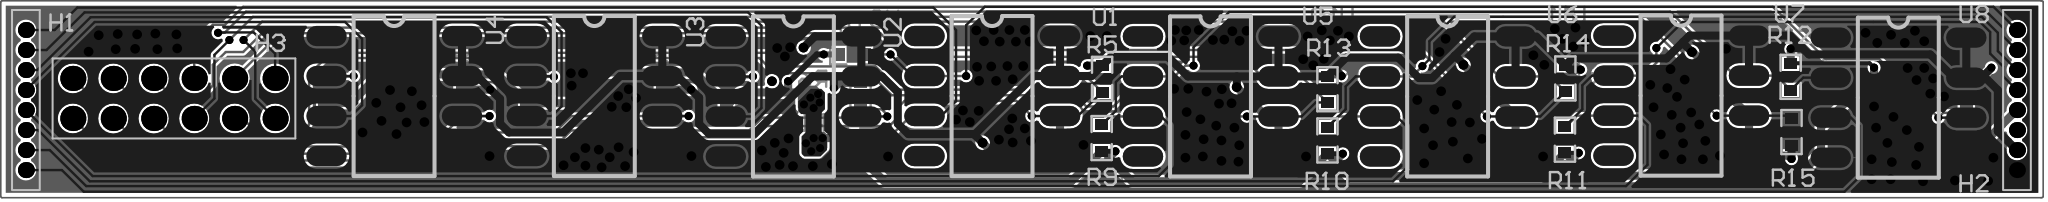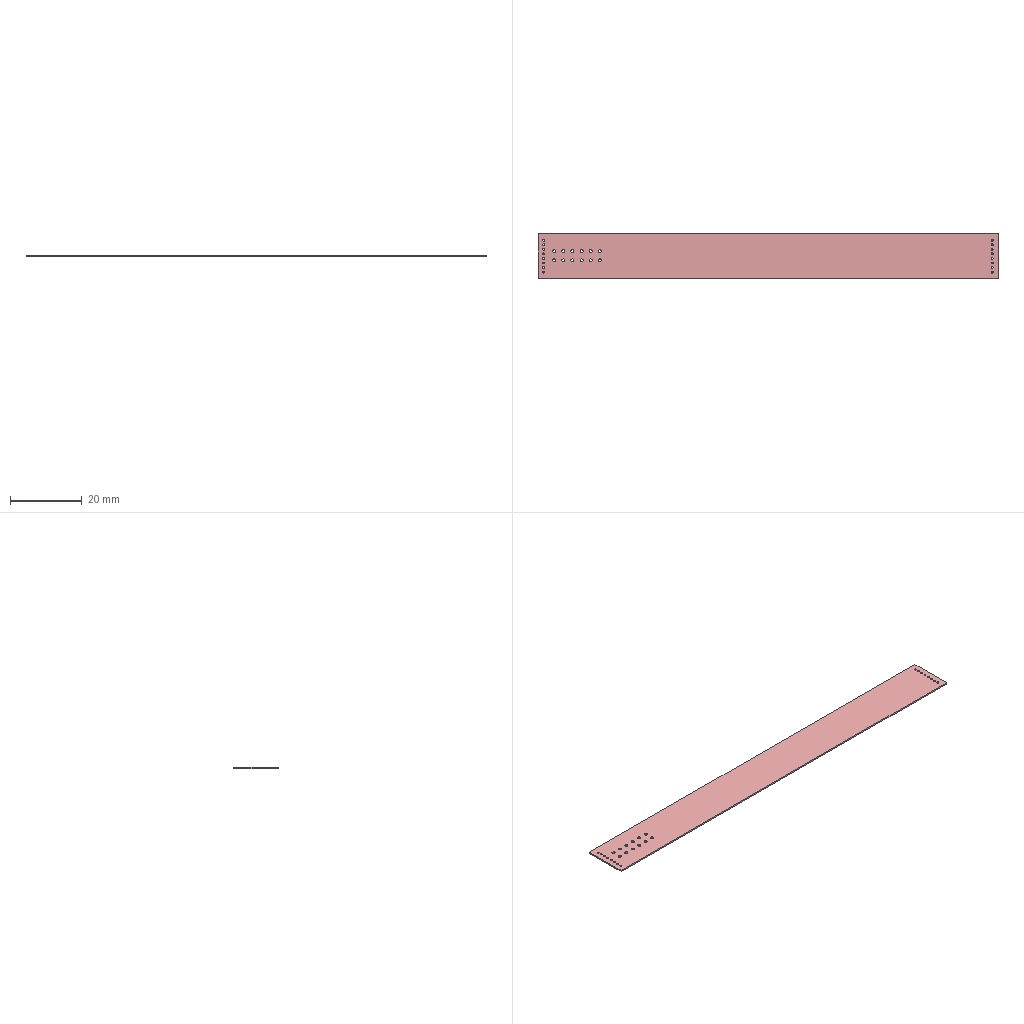Circuit board layout | Altium Designer | box 128.2 x 12.5 x 0.4 mm
Layer stack:
# Altium Designer layer stack of  (unit mm; dielectric type: 0 none, 1 core, 2 prepreg, 3 surface material)
index,name,kind,layer,copper_thickness_mm,dielectric_type,dielectric_thickness_mm,dielectric_material,dielectric_constant
0,Top Paste,other,,,,,,
1,Top Overlay,other,,,,,,
2,Top Solder,dielectric,,,3,0.0102,Solder Resist,3.5
3,Top Layer,copper,Top Layer,0.0356,,,,
4,Dielectric1,dielectric,,,0,0.32,FR-4,4.8
5,Bottom Layer,copper,Bottom Layer,0.0356,,,,
6,Bottom Solder,dielectric,,,3,0.0102,Solder Resist,3.5
7,Bottom Overlay,other,,,,,,
8,Bottom Paste,other,,,,,,
# drill layer pairs: low layer,high layer
drill_pair,Top Layer,Bottom Layer
Part placement:
Designator,Comment,Layer,Footprint,Center-X(mm),Center-Y(mm),Rotation
H1,Header8,TopLayer,PinHeader8_1.27mm,1.499,6.121,270
H2,Header8,TopLayer,PinHeader8_1.27mm,126.499,6.121,270
H3,Header6*2,TopLayer,PinHeader6*2_2.54mm,10.795,6.223,360
U1,6N137,TopLayer,6N137_SMD,62.166,6.375,360
U2,6N137,TopLayer,6N137_SMD,49.695,6.35,360
U3,6N137,TopLayer,6N137_SMD,37.198,6.375,360
U4,6N137,TopLayer,6N137_SMD,24.625,6.375,360
U5,6N137,TopLayer,6N137_SMD,75.882,6.35,360
U6,6N137,TopLayer,6N137_SMD,90.767,6.35,360
U7,6N137,TopLayer,6N137_SMD,105.423,6.401,360
U8,6N137,TopLayer,6N137_SMD,119.062,6.274,360
U9,6N137,BottomLayer,6N137_SMD,62.166,6.375,0
U10,6N137,BottomLayer,6N137_SMD,75.882,6.35,0
U11,6N137,BottomLayer,6N137_SMD,90.767,6.35,0
U12,6N137,BottomLayer,6N137_SMD,105.423,6.401,0
R1,470R,BottomLayer,0603,53.391,9.017,180
R2,470R,BottomLayer,0603,45.466,6.731,270
R3,470R,BottomLayer,0603,32.944,6.756,270
R4,470R,BottomLayer,0603,20.269,6.782,270
R5,4.7k,TopLayer,0603,69.063,7.468,270
R6,4.7k,BottomLayer,0603,53.899,6.375,270
R7,4.7k,BottomLayer,0603,41.453,5.944,270
R8,4.7k,BottomLayer,0603,28.88,5.944,270
R9,470R,TopLayer,0603,69.037,3.708,270
R10,470R,TopLayer,0603,83.21,3.556,270
R11,470R,TopLayer,0603,98.12,3.607,270
R12,470R,TopLayer,0603,112.293,7.595,90
R13,4.7k,TopLayer,0603,83.21,6.807,270
R14,4.7k,TopLayer,0603,98.146,7.493,270
R15,4.7k,TopLayer,0603,112.344,4.089,90
R16,4.7k,BottomLayer,0603,123.317,6.706,270
R17,470R,BottomLayer,0603,53.492,3.708,180
R18,470R,BottomLayer,0603,69.037,3.708,270
R19,470R,BottomLayer,0603,83.21,3.556,270
R20,470R,BottomLayer,0603,98.12,3.607,270
R21,4.7k,BottomLayer,0603,69.063,7.468,270
R22,4.7k,BottomLayer,0603,83.21,6.807,270
R23,4.7k,BottomLayer,0603,98.146,7.493,270
R24,4.7k,BottomLayer,0603,112.293,7.595,270
Pad and via stacks:
# Altium Designer via and pad stacks of  (unit mm). Each distinct definition once, with the count of objects using it.
# via: kind,start_layer,end_layer,hole_mm,diameter_mm,mode(0 simple;1 top-mid-bottom;2 full stack),diameter_per_layer,count,example_net
# pad: kind,layer,hole_mm,hole_type(0 round;1 square;2 slot),plating,top_size,top_shape(1 round;2 rect;3 octagon;9 rounded rect),mid_size,bottom_size,mode,footprint,size_per_layer,count,example
pad,Top Layer,0,0,plated,2.54x1.27,1,2.54x1.27,2.54x1.27,0,6N137_SMD,,64,U8.5
pad,Top Layer,0,0,plated,0.635x0.8128,2,0.635x0.8128,0.635x0.8128,0,0603,,16,R12.1
pad,Bottom Layer,0,0,plated,0.635x0.8128,2,0.635x0.8128,0.635x0.8128,0,0603,,32,R16.2
pad,Bottom Layer,0,0,plated,2.54x1.27,1,2.54x1.27,2.54x1.27,0,6N137_SMD,,32,U12.5
pad,Multi-Layer,0.5334,0,plated,1x1,1,1x1,1x1,0,PinHeader8_1.27mm,,16,H2.8
pad,Multi-Layer,0.8636,0,plated,1.575x1.575,1,1.575x1.575,1.575x1.575,0,PinHeader6*2_2.54mm,,12,H3.12
via,Top Layer,Bottom Layer,0.3048,0.508,0,,7,+5V_EXT
via,Top Layer,Bottom Layer,0.3048,0.6096,0,,191,GND_EXT
via,Top Layer,Bottom Layer,0.254,0.508,0,,37,+5V
Copper pours:
name,layer,net,type(0 solid;1 hatched;2 none)
Top Layer-No Net,Top Layer,GND_EXT,0
Top Layer-No Net,Top Layer,+5V,0
Top Layer-No Net,Top Layer,+5V,0
Top Layer-No Net,Bottom Layer,GND_EXT,0
Top Layer-No Net,Bottom Layer,+5V,0
Top Layer-No Net,Bottom Layer,+5V,0
Design rules, without the lines most boards share:
# Altium Designer design rules of  (exported by Altium Designer, unit mm)
# columns: name | kind | enabled | priority | scope1 | scope2 | descriptor | typed fields (field=value)
Clearance | 0 | enabled | 1 | All | All | Clearance Constraint (Gap=6mil) (All),(All) | gap=0.1524
PlaneConnect | 6 | enabled | 1 | All | All | Power Plane Connect Rule(Direct Connect )(Expansion=20mil) (Conductor Width=10mil) (Air Gap=10mil) (Entries=4) (All) | relief_conductor_width=0.254 relief_entries=4 relief_expansion=0.508
PlaneClearance | 12 | enabled | 1 | All | All | Power Plane Clearance (Clearance =30mil) (All) | clearance=0.762
PolygonConnect | 20 | enabled | 1 | All | All | Polygon Connect Rule(Direct Connect )(Conductor Width=6mil) (Relief Angle=90 Angle) (Entries=4) (Air Gap Width=10mil) (All),(All) | connect_style(0=relief,1=direct,2=none)=1 relief_conductor_width=0.1524 relief_entries=4
Width | 2 | enabled | 1 | All | All | Width Constraint (Min=6mil) (Max=40mil) (Preferred=6mil) (All) |
RoutingVias | 11 | enabled | 1 | All | All | Routing Via (MinHoleWidth=10mil) (MaxHoleWidth=12mil) (PreferredHoleWidth=12mil) (MinWidth=20mil) (MaxWidth=24mil) (PreferedWidth=24mil) (All) | via_min_hole=0.254 via_max_hole=0.3048 via_preferred_diameter=0.6096 via_preferred_hole=0.3048
PasteMaskExpansion | 14 | enabled | 1 | All | All | Paste Mask Expansion (Expansion =0mil) (All) | expansion=0
SolderMaskExpansion | 13 | enabled | 1 | All | All | Solder Mask Expansion (Expansion =4mil) (All) | expansion=0.1016
TestPointUsage | 44 | enabled | 1 | All | All | Fabrication Testpoint Usage (Valid =One Required, Allow multiple per net=No) (All) |
Testpoint | 43 | enabled | 1 | (IsPad And (OnTopLayer Or OnBottomLayer)) | All | Fabrication Testpoint Style (Under Component=Yes) ((IsPad And (OnTopLayer Or OnBottomLayer))) |
HoleSize | 42 | enabled | 1 | All | All | Hole Size Constraint (Min=8mil) (Max=100mil) (All) |
DiffPairsRouting | 51 | enabled | 1 | All | All | Differential Pairs Uncoupled Length using the Gap Constraints (Min=10mil) (Max=10mil) (Prefered=10mil)  and Width Constraints (Min=15mil) (Max=15mil) (Prefered=15mil) (All) |
HoleToHoleClearance | 52 | enabled | 1 | All | All | Hole To Hole Clearance (Gap=10mil) (All),(All) | gap=0.254
SilkscreenOverComponentPads | 54 | enabled | 1 | IsPad | All | Silk To Solder Mask (Clearance=10mil) (IsPad),(All) |